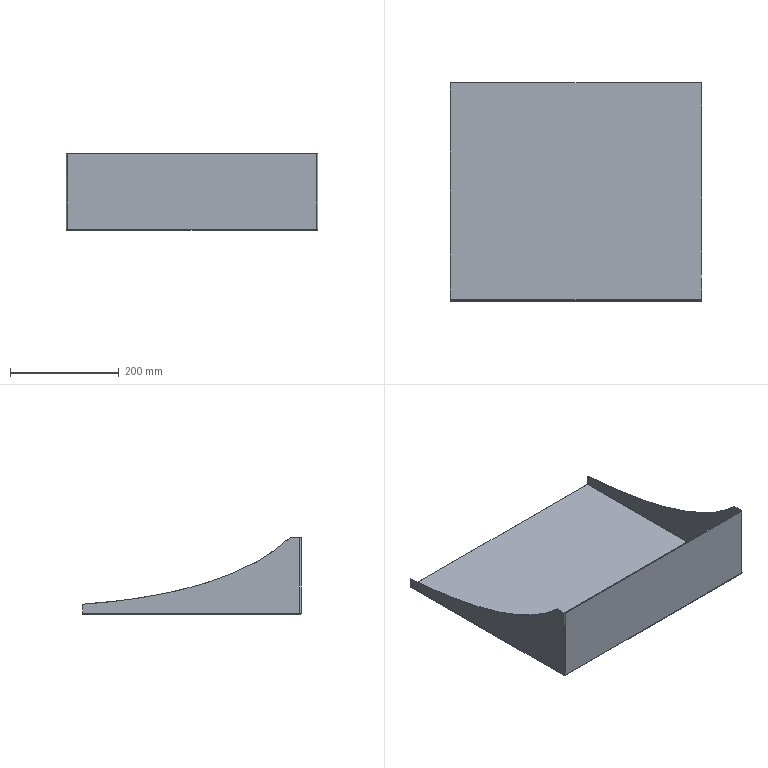Part | STEP file | Conveyor belt fixing plate | 1 solid | 34 faces | box 463 x 401.5 x 141.5 mm | volume 444630 mm3 | plane 26 | cylinder 6 | spline 2 | commonest cylinder face diameters 1.473 x3 4.473 x3